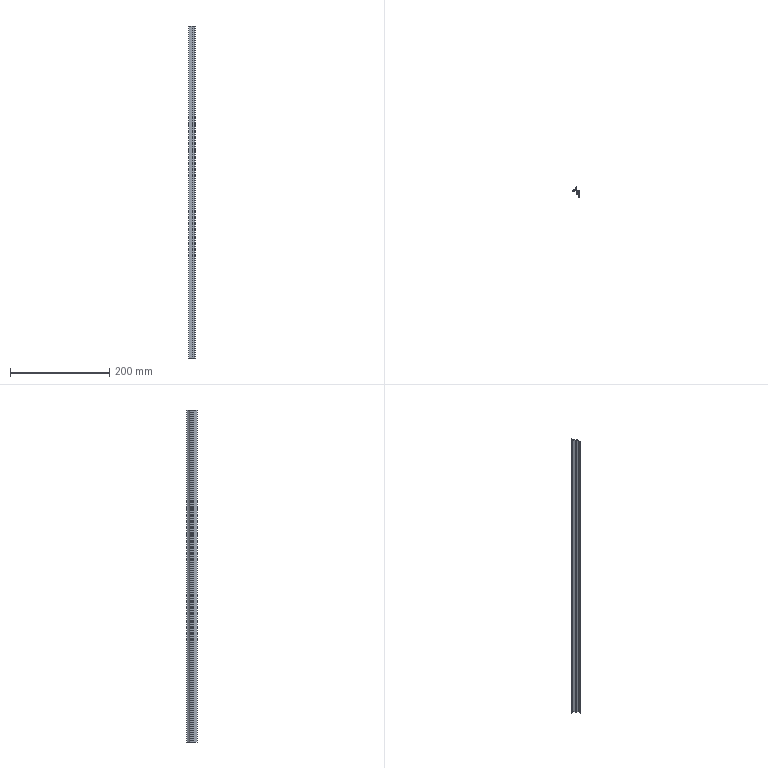Part | SolidWorks | features BaseBody 1, ICE 1, MoveFace 1 | 1 solid | 27 faces | box 14 x 20.3 x 670 mm | volume 34114 mm3 | plane 20 | cylinder 7 | commonest cylinder face diameters 0.387 x2 0.8 x2 0.4 x1 20 x1 22 x1
STEP:
#1=CARTESIAN_POINT('',(-5.304,-0.625,200.));
#2=VERTEX_POINT('',#1);
#3=CARTESIAN_POINT('',(-5.449,-0.8125,200.));
#4=VERTEX_POINT('',#3);
#5=CARTESIAN_POINT('',(-5.255,-0.8125,200.));
#6=DIRECTION('',(0.,0.,1.));
#7=DIRECTION('',(-1.,0.,0.));
#8=AXIS2_PLACEMENT_3D('',#5,#6,#7);
#9=CIRCLE('',#8,0.1937);
#10=EDGE_CURVE('',#2,#4,#9,.T.);
#11=ORIENTED_EDGE('',*,*,#10,.T.);
#12=CARTESIAN_POINT('',(-5.449,-0.8125,-470.));
#13=VERTEX_POINT('',#12);
#14=CARTESIAN_POINT('',(-5.449,-0.8125,230.));
#15=DIRECTION('',(0.,0.,-1.));
#16=VECTOR('',#15,1000.);
#17=LINE('',#14,#16);
#18=EDGE_CURVE('',#4,#13,#17,.T.);
#19=ORIENTED_EDGE('',*,*,#18,.T.);
#20=CARTESIAN_POINT('',(-5.304,-0.625,-470.));
#21=VERTEX_POINT('',#20);
#22=CARTESIAN_POINT('',(-5.255,-0.8125,-470.));
#23=DIRECTION('',(0.,0.,-1.));
#24=DIRECTION('',(1.,0.,0.));
#25=AXIS2_PLACEMENT_3D('',#22,#23,#24);
#26=CIRCLE('',#25,0.1937);
#27=EDGE_CURVE('',#13,#21,#26,.T.);
#28=ORIENTED_EDGE('',*,*,#27,.T.);
#29=CARTESIAN_POINT('',(-5.304,-0.625,230.));
#30=DIRECTION('',(0.,0.,-1.));
#31=VECTOR('',#30,1000.);
#32=LINE('',#29,#31);
#33=EDGE_CURVE('',#2,#21,#32,.T.);
#34=ORIENTED_EDGE('',*,*,#33,.F.);
#35=EDGE_LOOP('',(#11,#19,#28,#34));
#36=FACE_OUTER_BOUND('',#35,.T.);
#37=CARTESIAN_POINT('',(-5.255,-0.8125,230.));
#38=DIRECTION('',(0.,0.,-1.));
#39=DIRECTION('',(-1.,0.,0.));
#40=AXIS2_PLACEMENT_3D('',#37,#38,#39);
#41=CYLINDRICAL_SURFACE('',#40,0.1937);
#42=ADVANCED_FACE('',(#36),#41,.F.);
#43=CARTESIAN_POINT('',(5.,-1.,-470.));
#44=VERTEX_POINT('',#43);
#45=CARTESIAN_POINT('',(5.,-14.3,-470.));
#46=VERTEX_POINT('',#45);
#47=CARTESIAN_POINT('',(5.,29.623,-470.));
#48=DIRECTION('',(0.,-1.,0.));
#49=VECTOR('',#48,1000.);
#50=LINE('',#47,#49);
#51=EDGE_CURVE('',#44,#46,#50,.T.);
#52=ORIENTED_EDGE('',*,*,#51,.F.);
#53=CARTESIAN_POINT('',(5.,-1.,200.));
#54=VERTEX_POINT('',#53);
#55=CARTESIAN_POINT('',(5.,-1.,230.));
#56=DIRECTION('',(0.,0.,-1.));
#57=VECTOR('',#56,1000.);
#58=LINE('',#55,#57);
#59=EDGE_CURVE('',#54,#44,#58,.T.);
#60=ORIENTED_EDGE('',*,*,#59,.F.);
#61=CARTESIAN_POINT('',(5.,-14.3,200.));
#62=VERTEX_POINT('',#61);
#63=CARTESIAN_POINT('',(5.,-14.3,200.));
#64=DIRECTION('',(0.,1.,0.));
#65=VECTOR('',#64,1000.);
#66=LINE('',#63,#65);
#67=EDGE_CURVE('',#62,#54,#66,.T.);
#68=ORIENTED_EDGE('',*,*,#67,.F.);
#69=CARTESIAN_POINT('',(5.,-14.3,230.));
#70=DIRECTION('',(0.,0.,1.));
#71=VECTOR('',#70,1000.);
#72=LINE('',#69,#71);
#73=EDGE_CURVE('',#46,#62,#72,.T.);
#74=ORIENTED_EDGE('',*,*,#73,.F.);
#75=EDGE_LOOP('',(#52,#60,#68,#74));
#76=FACE_OUTER_BOUND('',#75,.T.);
#77=CARTESIAN_POINT('',(5.,-14.3,230.));
#78=DIRECTION('',(-1.,0.,0.));
#79=DIRECTION('',(0.,0.,1.));
#80=AXIS2_PLACEMENT_3D('',#77,#78,#79);
#81=PLANE('',#80);
#82=ADVANCED_FACE('',(#76),#81,.F.);
#83=CARTESIAN_POINT('',(-9.,-2.,-470.));
#84=VERTEX_POINT('',#83);
#85=CARTESIAN_POINT('',(-9.,-2.,200.));
#86=VERTEX_POINT('',#85);
#87=CARTESIAN_POINT('',(-9.,-2.,230.));
#88=DIRECTION('',(0.,0.,1.));
#89=VECTOR('',#88,1000.);
#90=LINE('',#87,#89);
#91=EDGE_CURVE('',#84,#86,#90,.T.);
#92=ORIENTED_EDGE('',*,*,#91,.F.);
#93=CARTESIAN_POINT('',(0.9,-2.,-470.));
#94=VERTEX_POINT('',#93);
#95=CARTESIAN_POINT('',(5.,-2.,-470.));
#96=DIRECTION('',(-1.,0.,0.));
#97=VECTOR('',#96,1000.);
#98=LINE('',#95,#97);
#99=EDGE_CURVE('',#94,#84,#98,.T.);
#100=ORIENTED_EDGE('',*,*,#99,.F.);
#101=CARTESIAN_POINT('',(0.9,-2.,200.));
#102=VERTEX_POINT('',#101);
#103=CARTESIAN_POINT('',(0.9,-2.,230.));
#104=DIRECTION('',(0.,0.,-1.));
#105=VECTOR('',#104,1000.);
#106=LINE('',#103,#105);
#107=EDGE_CURVE('',#102,#94,#106,.T.);
#108=ORIENTED_EDGE('',*,*,#107,.F.);
#109=CARTESIAN_POINT('',(5.,-2.,200.));
#110=DIRECTION('',(1.,0.,0.));
#111=VECTOR('',#110,1000.);
#112=LINE('',#109,#111);
#113=EDGE_CURVE('',#86,#102,#112,.T.);
#114=ORIENTED_EDGE('',*,*,#113,.F.);
#115=EDGE_LOOP('',(#92,#100,#108,#114));
#116=FACE_OUTER_BOUND('',#115,.T.);
#117=CARTESIAN_POINT('',(-9.,-2.,230.));
#118=DIRECTION('',(0.,1.,0.));
#119=DIRECTION('',(0.,0.,1.));
#120=AXIS2_PLACEMENT_3D('',#117,#118,#119);
#121=PLANE('',#120);
#122=ADVANCED_FACE('',(#116),#121,.F.);
#123=CARTESIAN_POINT('',(4.,-6.,200.));
#124=VERTEX_POINT('',#123);
#125=CARTESIAN_POINT('',(4.,-3.,200.));
#126=VERTEX_POINT('',#125);
#127=CARTESIAN_POINT('',(4.,29.623,200.));
#128=DIRECTION('',(0.,1.,0.));
#129=VECTOR('',#128,1000.);
#130=LINE('',#127,#129);
#131=EDGE_CURVE('',#124,#126,#130,.T.);
#132=ORIENTED_EDGE('',*,*,#131,.F.);
#133=CARTESIAN_POINT('',(1.,-6.,200.));
#134=VERTEX_POINT('',#133);
#135=CARTESIAN_POINT('',(5.,-6.,200.));
#136=DIRECTION('',(1.,0.,0.));
#137=VECTOR('',#136,1000.);
#138=LINE('',#135,#137);
#139=EDGE_CURVE('',#134,#124,#138,.T.);
#140=ORIENTED_EDGE('',*,*,#139,.F.);
#141=CARTESIAN_POINT('',(1.,-6.7,200.));
#142=VERTEX_POINT('',#141);
#143=CARTESIAN_POINT('',(1.,-6.,200.));
#144=DIRECTION('',(0.,-1.,0.));
#145=VECTOR('',#144,1000.);
#146=LINE('',#143,#145);
#147=EDGE_CURVE('',#134,#142,#146,.T.);
#148=ORIENTED_EDGE('',*,*,#147,.T.);
#149=CARTESIAN_POINT('',(-1.7,-6.7,200.));
#150=VERTEX_POINT('',#149);
#151=CARTESIAN_POINT('',(5.,-6.7,200.));
#152=DIRECTION('',(1.,0.,0.));
#153=VECTOR('',#152,1000.);
#154=LINE('',#151,#153);
#155=EDGE_CURVE('',#150,#142,#154,.T.);
#156=ORIENTED_EDGE('',*,*,#155,.F.);
#157=CARTESIAN_POINT('',(-1.7,-7.7,200.));
#158=VERTEX_POINT('',#157);
#159=CARTESIAN_POINT('',(-1.7,-6.7,200.));
#160=DIRECTION('',(0.,-1.,0.));
#161=VECTOR('',#160,1000.);
#162=LINE('',#159,#161);
#163=EDGE_CURVE('',#150,#158,#162,.T.);
#164=ORIENTED_EDGE('',*,*,#163,.T.);
#165=CARTESIAN_POINT('',(4.,-7.7,200.));
#166=VERTEX_POINT('',#165);
#167=CARTESIAN_POINT('',(5.,-7.7,200.));
#168=DIRECTION('',(-1.,0.,0.));
#169=VECTOR('',#168,1000.);
#170=LINE('',#167,#169);
#171=EDGE_CURVE('',#166,#158,#170,.T.);
#172=ORIENTED_EDGE('',*,*,#171,.F.);
#173=CARTESIAN_POINT('',(4.,-14.3,200.));
#174=VERTEX_POINT('',#173);
#175=CARTESIAN_POINT('',(4.,29.623,200.));
#176=DIRECTION('',(0.,1.,0.));
#177=VECTOR('',#176,1000.);
#178=LINE('',#175,#177);
#179=EDGE_CURVE('',#174,#166,#178,.T.);
#180=ORIENTED_EDGE('',*,*,#179,.F.);
#181=CARTESIAN_POINT('',(5.,-14.3,200.));
#182=DIRECTION('',(-1.,0.,0.));
#183=VECTOR('',#182,1000.);
#184=LINE('',#181,#183);
#185=EDGE_CURVE('',#62,#174,#184,.T.);
#186=ORIENTED_EDGE('',*,*,#185,.F.);
#187=ORIENTED_EDGE('',*,*,#67,.T.);
#188=CARTESIAN_POINT('',(-5.207,-1.,200.));
#189=VERTEX_POINT('',#188);
#190=CARTESIAN_POINT('',(5.,-1.,200.));
#191=DIRECTION('',(1.,0.,0.));
#192=VECTOR('',#191,1000.);
#193=LINE('',#190,#192);
#194=EDGE_CURVE('',#189,#54,#193,.T.);
#195=ORIENTED_EDGE('',*,*,#194,.F.);
#196=CARTESIAN_POINT('',(-5.255,-0.8125,200.));
#197=DIRECTION('',(0.,0.,1.));
#198=DIRECTION('',(-1.,0.,0.));
#199=AXIS2_PLACEMENT_3D('',#196,#197,#198);
#200=CIRCLE('',#199,0.1937);
#201=EDGE_CURVE('',#4,#189,#200,.T.);
#202=ORIENTED_EDGE('',*,*,#201,.F.);
#203=ORIENTED_EDGE('',*,*,#10,.F.);
#204=CARTESIAN_POINT('',(-1.368,3.063,200.));
#205=VERTEX_POINT('',#204);
#206=CARTESIAN_POINT('',(-10.628,9.,200.));
#207=DIRECTION('',(0.,0.,1.));
#208=DIRECTION('',(-1.,0.,0.));
#209=AXIS2_PLACEMENT_3D('',#206,#207,#208);
#210=CIRCLE('',#209,11.);
#211=EDGE_CURVE('',#2,#205,#210,.T.);
#212=ORIENTED_EDGE('',*,*,#211,.T.);
#213=CARTESIAN_POINT('',(-1.,2.955,200.));
#214=VERTEX_POINT('',#213);
#215=CARTESIAN_POINT('',(-1.2,2.955,200.));
#216=DIRECTION('',(0.,0.,1.));
#217=DIRECTION('',(-1.,0.,0.));
#218=AXIS2_PLACEMENT_3D('',#215,#216,#217);
#219=CIRCLE('',#218,0.2);
#220=EDGE_CURVE('',#214,#205,#219,.T.);
#221=ORIENTED_EDGE('',*,*,#220,.F.);
#222=CARTESIAN_POINT('',(-1.,1.5,200.));
#223=VERTEX_POINT('',#222);
#224=CARTESIAN_POINT('',(-1.,2.955,200.));
#225=DIRECTION('',(0.,1.,0.));
#226=VECTOR('',#225,1000.);
#227=LINE('',#224,#226);
#228=EDGE_CURVE('',#223,#214,#227,.T.);
#229=ORIENTED_EDGE('',*,*,#228,.F.);
#230=CARTESIAN_POINT('',(0.,1.5,200.));
#231=VERTEX_POINT('',#230);
#232=CARTESIAN_POINT('',(-1.,1.5,200.));
#233=DIRECTION('',(-1.,0.,0.));
#234=VECTOR('',#233,1000.);
#235=LINE('',#232,#234);
#236=EDGE_CURVE('',#231,#223,#235,.T.);
#237=ORIENTED_EDGE('',*,*,#236,.F.);
#238=CARTESIAN_POINT('',(0.,6.,200.));
#239=VERTEX_POINT('',#238);
#240=CARTESIAN_POINT('',(0.,1.5,200.));
#241=DIRECTION('',(0.,-1.,0.));
#242=VECTOR('',#241,1000.);
#243=LINE('',#240,#242);
#244=EDGE_CURVE('',#239,#231,#243,.T.);
#245=ORIENTED_EDGE('',*,*,#244,.F.);
#246=CARTESIAN_POINT('',(-0.8,6.,200.));
#247=VERTEX_POINT('',#246);
#248=CARTESIAN_POINT('',(0.,6.,200.));
#249=DIRECTION('',(1.,0.,0.));
#250=VECTOR('',#249,1000.);
#251=LINE('',#248,#250);
#252=EDGE_CURVE('',#247,#239,#251,.T.);
#253=ORIENTED_EDGE('',*,*,#252,.F.);
#254=CARTESIAN_POINT('',(-1.178,5.731,200.));
#255=VERTEX_POINT('',#254);
#256=CARTESIAN_POINT('',(-0.8,5.6,200.));
#257=DIRECTION('',(0.,0.,1.));
#258=DIRECTION('',(-1.,0.,0.));
#259=AXIS2_PLACEMENT_3D('',#256,#257,#258);
#260=CIRCLE('',#259,0.4);
#261=EDGE_CURVE('',#247,#255,#260,.T.);
#262=ORIENTED_EDGE('',*,*,#261,.T.);
#263=CARTESIAN_POINT('',(-8.678,-0.8077,200.));
#264=VERTEX_POINT('',#263);
#265=CARTESIAN_POINT('',(-10.628,9.,200.));
#266=DIRECTION('',(0.,0.,1.));
#267=DIRECTION('',(-1.,0.,0.));
#268=AXIS2_PLACEMENT_3D('',#265,#266,#267);
#269=CIRCLE('',#268,10.);
#270=EDGE_CURVE('',#264,#255,#269,.T.);
#271=ORIENTED_EDGE('',*,*,#270,.F.);
#272=CARTESIAN_POINT('',(-9.,-1.2,200.));
#273=VERTEX_POINT('',#272);
#274=CARTESIAN_POINT('',(-8.6,-1.2,200.));
#275=DIRECTION('',(0.,0.,1.));
#276=DIRECTION('',(-1.,0.,0.));
#277=AXIS2_PLACEMENT_3D('',#274,#275,#276);
#278=CIRCLE('',#277,0.4);
#279=EDGE_CURVE('',#264,#273,#278,.T.);
#280=ORIENTED_EDGE('',*,*,#279,.T.);
#281=CARTESIAN_POINT('',(-9.,8.,200.));
#282=DIRECTION('',(0.,-1.,0.));
#283=VECTOR('',#282,1000.);
#284=LINE('',#281,#283);
#285=EDGE_CURVE('',#273,#86,#284,.T.);
#286=ORIENTED_EDGE('',*,*,#285,.T.);
#287=ORIENTED_EDGE('',*,*,#113,.T.);
#288=CARTESIAN_POINT('',(0.9,-3.,200.));
#289=VERTEX_POINT('',#288);
#290=CARTESIAN_POINT('',(0.9,29.623,200.));
#291=DIRECTION('',(0.,1.,0.));
#292=VECTOR('',#291,1000.);
#293=LINE('',#290,#292);
#294=EDGE_CURVE('',#289,#102,#293,.T.);
#295=ORIENTED_EDGE('',*,*,#294,.F.);
#296=CARTESIAN_POINT('',(5.,-3.,200.));
#297=DIRECTION('',(-1.,0.,0.));
#298=VECTOR('',#297,1000.);
#299=LINE('',#296,#298);
#300=EDGE_CURVE('',#126,#289,#299,.T.);
#301=ORIENTED_EDGE('',*,*,#300,.F.);
#302=EDGE_LOOP('',(#132,#140,#148,#156,#164,#172,#180,#186,#187,#195,#202,#203,#212,#221,#229,#237,#245,#253,#262,#271,#280,#286,#287,#295,#301));
#303=FACE_OUTER_BOUND('',#302,.T.);
#304=CARTESIAN_POINT('',(5.,29.623,200.));
#305=DIRECTION('',(0.,0.,-1.));
#306=DIRECTION('',(-1.,0.,0.));
#307=AXIS2_PLACEMENT_3D('',#304,#305,#306);
#308=PLANE('',#307);
#309=ADVANCED_FACE('',(#303),#308,.F.);
#310=ORIENTED_EDGE('',*,*,#185,.T.);
#311=CARTESIAN_POINT('',(4.,-14.3,-470.));
#312=VERTEX_POINT('',#311);
#313=CARTESIAN_POINT('',(4.,-14.3,230.));
#314=DIRECTION('',(0.,0.,1.));
#315=VECTOR('',#314,1000.);
#316=LINE('',#313,#315);
#317=EDGE_CURVE('',#312,#174,#316,.T.);
#318=ORIENTED_EDGE('',*,*,#317,.F.);
#319=CARTESIAN_POINT('',(5.,-14.3,-470.));
#320=DIRECTION('',(-1.,0.,0.));
#321=VECTOR('',#320,1000.);
#322=LINE('',#319,#321);
#323=EDGE_CURVE('',#46,#312,#322,.T.);
#324=ORIENTED_EDGE('',*,*,#323,.F.);
#325=ORIENTED_EDGE('',*,*,#73,.T.);
#326=EDGE_LOOP('',(#310,#318,#324,#325));
#327=FACE_OUTER_BOUND('',#326,.T.);
#328=CARTESIAN_POINT('',(4.,-14.3,230.));
#329=DIRECTION('',(0.,1.,0.));
#330=DIRECTION('',(0.,0.,1.));
#331=AXIS2_PLACEMENT_3D('',#328,#329,#330);
#332=PLANE('',#331);
#333=ADVANCED_FACE('',(#327),#332,.F.);
#334=ORIENTED_EDGE('',*,*,#51,.T.);
#335=ORIENTED_EDGE('',*,*,#323,.T.);
#336=CARTESIAN_POINT('',(4.,-7.7,-470.));
#337=VERTEX_POINT('',#336);
#338=CARTESIAN_POINT('',(4.,-7.7,-470.));
#339=DIRECTION('',(0.,-1.,0.));
#340=VECTOR('',#339,1000.);
#341=LINE('',#338,#340);
#342=EDGE_CURVE('',#337,#312,#341,.T.);
#343=ORIENTED_EDGE('',*,*,#342,.F.);
#344=CARTESIAN_POINT('',(-1.7,-7.7,-470.));
#345=VERTEX_POINT('',#344);
#346=CARTESIAN_POINT('',(-1.7,-7.7,-470.));
#347=DIRECTION('',(1.,0.,0.));
#348=VECTOR('',#347,1000.);
#349=LINE('',#346,#348);
#350=EDGE_CURVE('',#345,#337,#349,.T.);
#351=ORIENTED_EDGE('',*,*,#350,.F.);
#352=CARTESIAN_POINT('',(-1.7,-6.7,-470.));
#353=VERTEX_POINT('',#352);
#354=CARTESIAN_POINT('',(-1.7,29.623,-470.));
#355=DIRECTION('',(0.,1.,0.));
#356=VECTOR('',#355,1000.);
#357=LINE('',#354,#356);
#358=EDGE_CURVE('',#345,#353,#357,.T.);
#359=ORIENTED_EDGE('',*,*,#358,.T.);
#360=CARTESIAN_POINT('',(1.,-6.7,-470.));
#361=VERTEX_POINT('',#360);
#362=CARTESIAN_POINT('',(1.,-6.7,-470.));
#363=DIRECTION('',(-1.,0.,0.));
#364=VECTOR('',#363,1000.);
#365=LINE('',#362,#364);
#366=EDGE_CURVE('',#361,#353,#365,.T.);
#367=ORIENTED_EDGE('',*,*,#366,.F.);
#368=CARTESIAN_POINT('',(1.,-6.,-470.));
#369=VERTEX_POINT('',#368);
#370=CARTESIAN_POINT('',(1.,29.623,-470.));
#371=DIRECTION('',(0.,1.,0.));
#372=VECTOR('',#371,1000.);
#373=LINE('',#370,#372);
#374=EDGE_CURVE('',#361,#369,#373,.T.);
#375=ORIENTED_EDGE('',*,*,#374,.T.);
#376=CARTESIAN_POINT('',(4.,-6.,-470.));
#377=VERTEX_POINT('',#376);
#378=CARTESIAN_POINT('',(4.,-6.,-470.));
#379=DIRECTION('',(-1.,0.,0.));
#380=VECTOR('',#379,1000.);
#381=LINE('',#378,#380);
#382=EDGE_CURVE('',#377,#369,#381,.T.);
#383=ORIENTED_EDGE('',*,*,#382,.F.);
#384=CARTESIAN_POINT('',(4.,-3.,-470.));
#385=VERTEX_POINT('',#384);
#386=CARTESIAN_POINT('',(4.,-3.,-470.));
#387=DIRECTION('',(0.,-1.,0.));
#388=VECTOR('',#387,1000.);
#389=LINE('',#386,#388);
#390=EDGE_CURVE('',#385,#377,#389,.T.);
#391=ORIENTED_EDGE('',*,*,#390,.F.);
#392=CARTESIAN_POINT('',(0.9,-3.,-470.));
#393=VERTEX_POINT('',#392);
#394=CARTESIAN_POINT('',(0.9,-3.,-470.));
#395=DIRECTION('',(1.,0.,0.));
#396=VECTOR('',#395,1000.);
#397=LINE('',#394,#396);
#398=EDGE_CURVE('',#393,#385,#397,.T.);
#399=ORIENTED_EDGE('',*,*,#398,.F.);
#400=CARTESIAN_POINT('',(0.9,-2.,-470.));
#401=DIRECTION('',(0.,-1.,0.));
#402=VECTOR('',#401,1000.);
#403=LINE('',#400,#402);
#404=EDGE_CURVE('',#94,#393,#403,.T.);
#405=ORIENTED_EDGE('',*,*,#404,.F.);
#406=ORIENTED_EDGE('',*,*,#99,.T.);
#407=CARTESIAN_POINT('',(-9.,-1.2,-470.));
#408=VERTEX_POINT('',#407);
#409=CARTESIAN_POINT('',(-9.,-1.2,-470.));
#410=DIRECTION('',(0.,-1.,0.));
#411=VECTOR('',#410,1000.);
#412=LINE('',#409,#411);
#413=EDGE_CURVE('',#408,#84,#412,.T.);
#414=ORIENTED_EDGE('',*,*,#413,.F.);
#415=CARTESIAN_POINT('',(-8.678,-0.8077,-470.));
#416=VERTEX_POINT('',#415);
#417=CARTESIAN_POINT('',(-8.6,-1.2,-470.));
#418=DIRECTION('',(0.,0.,-1.));
#419=DIRECTION('',(1.,0.,0.));
#420=AXIS2_PLACEMENT_3D('',#417,#418,#419);
#421=CIRCLE('',#420,0.4);
#422=EDGE_CURVE('',#408,#416,#421,.T.);
#423=ORIENTED_EDGE('',*,*,#422,.T.);
#424=CARTESIAN_POINT('',(-1.178,5.731,-470.));
#425=VERTEX_POINT('',#424);
#426=CARTESIAN_POINT('',(-10.628,9.,-470.));
#427=DIRECTION('',(0.,0.,-1.));
#428=DIRECTION('',(1.,0.,0.));
#429=AXIS2_PLACEMENT_3D('',#426,#427,#428);
#430=CIRCLE('',#429,10.);
#431=EDGE_CURVE('',#425,#416,#430,.T.);
#432=ORIENTED_EDGE('',*,*,#431,.F.);
#433=CARTESIAN_POINT('',(-0.8,6.,-470.));
#434=VERTEX_POINT('',#433);
#435=CARTESIAN_POINT('',(-0.8,5.6,-470.));
#436=DIRECTION('',(0.,0.,-1.));
#437=DIRECTION('',(1.,0.,0.));
#438=AXIS2_PLACEMENT_3D('',#435,#436,#437);
#439=CIRCLE('',#438,0.4);
#440=EDGE_CURVE('',#425,#434,#439,.T.);
#441=ORIENTED_EDGE('',*,*,#440,.T.);
#442=CARTESIAN_POINT('',(0.,6.,-470.));
#443=VERTEX_POINT('',#442);
#444=CARTESIAN_POINT('',(0.,6.,-470.));
#445=DIRECTION('',(-1.,0.,0.));
#446=VECTOR('',#445,1000.);
#447=LINE('',#444,#446);
#448=EDGE_CURVE('',#443,#434,#447,.T.);
#449=ORIENTED_EDGE('',*,*,#448,.F.);
#450=CARTESIAN_POINT('',(0.,1.5,-470.));
#451=VERTEX_POINT('',#450);
#452=CARTESIAN_POINT('',(0.,1.5,-470.));
#453=DIRECTION('',(0.,1.,0.));
#454=VECTOR('',#453,1000.);
#455=LINE('',#452,#454);
#456=EDGE_CURVE('',#451,#443,#455,.T.);
#457=ORIENTED_EDGE('',*,*,#456,.F.);
#458=CARTESIAN_POINT('',(-1.,1.5,-470.));
#459=VERTEX_POINT('',#458);
#460=CARTESIAN_POINT('',(-1.,1.5,-470.));
#461=DIRECTION('',(1.,0.,0.));
#462=VECTOR('',#461,1000.);
#463=LINE('',#460,#462);
#464=EDGE_CURVE('',#459,#451,#463,.T.);
#465=ORIENTED_EDGE('',*,*,#464,.F.);
#466=CARTESIAN_POINT('',(-1.,2.955,-470.));
#467=VERTEX_POINT('',#466);
#468=CARTESIAN_POINT('',(-1.,2.955,-470.));
#469=DIRECTION('',(0.,-1.,0.));
#470=VECTOR('',#469,1000.);
#471=LINE('',#468,#470);
#472=EDGE_CURVE('',#467,#459,#471,.T.);
#473=ORIENTED_EDGE('',*,*,#472,.F.);
#474=CARTESIAN_POINT('',(-1.368,3.063,-470.));
#475=VERTEX_POINT('',#474);
#476=CARTESIAN_POINT('',(-1.2,2.955,-470.));
#477=DIRECTION('',(0.,0.,-1.));
#478=DIRECTION('',(1.,0.,0.));
#479=AXIS2_PLACEMENT_3D('',#476,#477,#478);
#480=CIRCLE('',#479,0.2);
#481=EDGE_CURVE('',#475,#467,#480,.T.);
#482=ORIENTED_EDGE('',*,*,#481,.F.);
#483=CARTESIAN_POINT('',(-10.628,9.,-470.));
#484=DIRECTION('',(0.,0.,-1.));
#485=DIRECTION('',(1.,0.,0.));
#486=AXIS2_PLACEMENT_3D('',#483,#484,#485);
#487=CIRCLE('',#486,11.);
#488=EDGE_CURVE('',#475,#21,#487,.T.);
#489=ORIENTED_EDGE('',*,*,#488,.T.);
#490=ORIENTED_EDGE('',*,*,#27,.F.);
#491=CARTESIAN_POINT('',(-5.207,-1.,-470.));
#492=VERTEX_POINT('',#491);
#493=CARTESIAN_POINT('',(-5.255,-0.8125,-470.));
#494=DIRECTION('',(0.,0.,-1.));
#495=DIRECTION('',(1.,0.,0.));
#496=AXIS2_PLACEMENT_3D('',#493,#494,#495);
#497=CIRCLE('',#496,0.1937);
#498=EDGE_CURVE('',#492,#13,#497,.T.);
#499=ORIENTED_EDGE('',*,*,#498,.F.);
#500=CARTESIAN_POINT('',(5.,-1.,-470.));
#501=DIRECTION('',(-1.,0.,0.));
#502=VECTOR('',#501,1000.);
#503=LINE('',#500,#502);
#504=EDGE_CURVE('',#44,#492,#503,.T.);
#505=ORIENTED_EDGE('',*,*,#504,.F.);
#506=EDGE_LOOP('',(#334,#335,#343,#351,#359,#367,#375,#383,#391,#399,#405,#406,#414,#423,#432,#441,#449,#457,#465,#473,#482,#489,#490,#499,#505));
#507=FACE_OUTER_BOUND('',#506,.T.);
#508=CARTESIAN_POINT('',(5.,29.623,-470.));
#509=DIRECTION('',(0.,0.,1.));
#510=DIRECTION('',(1.,0.,0.));
#511=AXIS2_PLACEMENT_3D('',#508,#509,#510);
#512=PLANE('',#511);
#513=ADVANCED_FACE('',(#507),#512,.F.);
#514=ORIENTED_EDGE('',*,*,#59,.T.);
#515=ORIENTED_EDGE('',*,*,#504,.T.);
#516=CARTESIAN_POINT('',(-5.207,-1.,230.));
#517=DIRECTION('',(0.,0.,-1.));
#518=VECTOR('',#517,1000.);
#519=LINE('',#516,#518);
#520=EDGE_CURVE('',#189,#492,#519,.T.);
#521=ORIENTED_EDGE('',*,*,#520,.F.);
#522=ORIENTED_EDGE('',*,*,#194,.T.);
#523=EDGE_LOOP('',(#514,#515,#521,#522));
#524=FACE_OUTER_BOUND('',#523,.T.);
#525=CARTESIAN_POINT('',(5.,-1.,230.));
#526=DIRECTION('',(0.,-1.,0.));
#527=DIRECTION('',(0.,0.,-1.));
#528=AXIS2_PLACEMENT_3D('',#525,#526,#527);
#529=PLANE('',#528);
#530=ADVANCED_FACE('',(#524),#529,.F.);
#531=CARTESIAN_POINT('',(-9.,-1.2,230.));
#532=DIRECTION('',(0.,0.,1.));
#533=VECTOR('',#532,1000.);
#534=LINE('',#531,#533);
#535=EDGE_CURVE('',#408,#273,#534,.T.);
#536=ORIENTED_EDGE('',*,*,#535,.F.);
#537=ORIENTED_EDGE('',*,*,#413,.T.);
#538=ORIENTED_EDGE('',*,*,#91,.T.);
#539=ORIENTED_EDGE('',*,*,#285,.F.);
#540=EDGE_LOOP('',(#536,#537,#538,#539));
#541=FACE_OUTER_BOUND('',#540,.T.);
#542=CARTESIAN_POINT('',(-9.,-1.2,230.));
#543=DIRECTION('',(1.,0.,0.));
#544=DIRECTION('',(0.,0.,-1.));
#545=AXIS2_PLACEMENT_3D('',#542,#543,#544);
#546=PLANE('',#545);
#547=ADVANCED_FACE('',(#541),#546,.F.);
#548=ORIENTED_EDGE('',*,*,#294,.T.);
#549=ORIENTED_EDGE('',*,*,#107,.T.);
#550=ORIENTED_EDGE('',*,*,#404,.T.);
#551=CARTESIAN_POINT('',(0.9,-3.,230.));
#552=DIRECTION('',(0.,0.,-1.));
#553=VECTOR('',#552,1000.);
#554=LINE('',#551,#553);
#555=EDGE_CURVE('',#289,#393,#554,.T.);
#556=ORIENTED_EDGE('',*,*,#555,.F.);
#557=EDGE_LOOP('',(#548,#549,#550,#556));
#558=FACE_OUTER_BOUND('',#557,.T.);
#559=CARTESIAN_POINT('',(0.9,-2.,230.));
#560=DIRECTION('',(1.,0.,0.));
#561=DIRECTION('',(0.,0.,-1.));
#562=AXIS2_PLACEMENT_3D('',#559,#560,#561);
#563=PLANE('',#562);
#564=ADVANCED_FACE('',(#558),#563,.F.);
#565=ORIENTED_EDGE('',*,*,#300,.T.);
#566=ORIENTED_EDGE('',*,*,#555,.T.);
#567=ORIENTED_EDGE('',*,*,#398,.T.);
#568=CARTESIAN_POINT('',(4.,-3.,230.));
#569=DIRECTION('',(0.,0.,-1.));
#570=VECTOR('',#569,1000.);
#571=LINE('',#568,#570);
#572=EDGE_CURVE('',#126,#385,#571,.T.);
#573=ORIENTED_EDGE('',*,*,#572,.F.);
#574=EDGE_LOOP('',(#565,#566,#567,#573));
#575=FACE_OUTER_BOUND('',#574,.T.);
#576=CARTESIAN_POINT('',(0.9,-3.,230.));
#577=DIRECTION('',(0.,1.,0.));
#578=DIRECTION('',(0.,0.,1.));
#579=AXIS2_PLACEMENT_3D('',#576,#577,#578);
#580=PLANE('',#579);
#581=ADVANCED_FACE('',(#575),#580,.F.);
#582=ORIENTED_EDGE('',*,*,#131,.T.);
#583=ORIENTED_EDGE('',*,*,#572,.T.);
#584=ORIENTED_EDGE('',*,*,#390,.T.);
#585=CARTESIAN_POINT('',(4.,-6.,230.));
#586=DIRECTION('',(0.,0.,-1.));
#587=VECTOR('',#586,1000.);
#588=LINE('',#585,#587);
#589=EDGE_CURVE('',#124,#377,#588,.T.);
#590=ORIENTED_EDGE('',*,*,#589,.F.);
#591=EDGE_LOOP('',(#582,#583,#584,#590));
#592=FACE_OUTER_BOUND('',#591,.T.);
#593=CARTESIAN_POINT('',(4.,-3.,230.));
#594=DIRECTION('',(1.,0.,0.));
#595=DIRECTION('',(0.,0.,-1.));
#596=AXIS2_PLACEMENT_3D('',#593,#594,#595);
#597=PLANE('',#596);
#598=ADVANCED_FACE('',(#592),#597,.F.);
#599=ORIENTED_EDGE('',*,*,#139,.T.);
#600=ORIENTED_EDGE('',*,*,#589,.T.);
#601=ORIENTED_EDGE('',*,*,#382,.T.);
#602=CARTESIAN_POINT('',(1.,-6.,230.));
#603=DIRECTION('',(0.,0.,-1.));
#604=VECTOR('',#603,1000.);
#605=LINE('',#602,#604);
#606=EDGE_CURVE('',#134,#369,#605,.T.);
#607=ORIENTED_EDGE('',*,*,#606,.F.);
#608=EDGE_LOOP('',(#599,#600,#601,#607));
#609=FACE_OUTER_BOUND('',#608,.T.);
#610=CARTESIAN_POINT('',(4.,-6.,230.));
#611=DIRECTION('',(0.,-1.,0.));
#612=DIRECTION('',(0.,0.,-1.));
#613=AXIS2_PLACEMENT_3D('',#610,#611,#612);
#614=PLANE('',#613);
#615=ADVANCED_FACE('',(#609),#614,.F.);
#616=ORIENTED_EDGE('',*,*,#155,.T.);
#617=CARTESIAN_POINT('',(1.,-6.7,230.));
#618=DIRECTION('',(0.,0.,1.));
#619=VECTOR('',#618,1000.);
#620=LINE('',#617,#619);
#621=EDGE_CURVE('',#361,#142,#620,.T.);
#622=ORIENTED_EDGE('',*,*,#621,.F.);
#623=ORIENTED_EDGE('',*,*,#366,.T.);
#624=CARTESIAN_POINT('',(-1.7,-6.7,230.));
#625=DIRECTION('',(0.,0.,-1.));
#626=VECTOR('',#625,1000.);
#627=LINE('',#624,#626);
#628=EDGE_CURVE('',#150,#353,#627,.T.);
#629=ORIENTED_EDGE('',*,*,#628,.F.);
#630=EDGE_LOOP('',(#616,#622,#623,#629));
#631=FACE_OUTER_BOUND('',#630,.T.);
#632=CARTESIAN_POINT('',(1.,-6.7,230.));
#633=DIRECTION('',(0.,-1.,0.));
#634=DIRECTION('',(0.,0.,-1.));
#635=AXIS2_PLACEMENT_3D('',#632,#633,#634);
#636=PLANE('',#635);
#637=ADVANCED_FACE('',(#631),#636,.F.);
#638=ORIENTED_EDGE('',*,*,#171,.T.);
#639=CARTESIAN_POINT('',(-1.7,-7.7,230.));
#640=DIRECTION('',(0.,0.,1.));
#641=VECTOR('',#640,1000.);
#642=LINE('',#639,#641);
#643=EDGE_CURVE('',#345,#158,#642,.T.);
#644=ORIENTED_EDGE('',*,*,#643,.F.);
#645=ORIENTED_EDGE('',*,*,#350,.T.);
#646=CARTESIAN_POINT('',(4.,-7.7,230.));
#647=DIRECTION('',(0.,0.,-1.));
#648=VECTOR('',#647,1000.);
#649=LINE('',#646,#648);
#650=EDGE_CURVE('',#166,#337,#649,.T.);
#651=ORIENTED_EDGE('',*,*,#650,.F.);
#652=EDGE_LOOP('',(#638,#644,#645,#651));
#653=FACE_OUTER_BOUND('',#652,.T.);
#654=CARTESIAN_POINT('',(-1.7,-7.7,230.));
#655=DIRECTION('',(0.,1.,0.));
#656=DIRECTION('',(0.,0.,1.));
#657=AXIS2_PLACEMENT_3D('',#654,#655,#656);
#658=PLANE('',#657);
#659=ADVANCED_FACE('',(#653),#658,.F.);
#660=ORIENTED_EDGE('',*,*,#179,.T.);
#661=ORIENTED_EDGE('',*,*,#650,.T.);
#662=ORIENTED_EDGE('',*,*,#342,.T.);
#663=ORIENTED_EDGE('',*,*,#317,.T.);
#664=EDGE_LOOP('',(#660,#661,#662,#663));
#665=FACE_OUTER_BOUND('',#664,.T.);
#666=CARTESIAN_POINT('',(4.,-7.7,230.));
#667=DIRECTION('',(1.,0.,0.));
#668=DIRECTION('',(0.,0.,-1.));
#669=AXIS2_PLACEMENT_3D('',#666,#667,#668);
#670=PLANE('',#669);
#671=ADVANCED_FACE('',(#665),#670,.F.);
#672=ORIENTED_EDGE('',*,*,#18,.F.);
#673=ORIENTED_EDGE('',*,*,#201,.T.);
#674=ORIENTED_EDGE('',*,*,#520,.T.);
#675=ORIENTED_EDGE('',*,*,#498,.T.);
#676=EDGE_LOOP('',(#672,#673,#674,#675));
#677=FACE_OUTER_BOUND('',#676,.T.);
#678=CARTESIAN_POINT('',(-5.255,-0.8125,230.));
#679=DIRECTION('',(0.,0.,-1.));
#680=DIRECTION('',(-1.,0.,0.));
#681=AXIS2_PLACEMENT_3D('',#678,#679,#680);
#682=CYLINDRICAL_SURFACE('',#681,0.1937);
#683=ADVANCED_FACE('',(#677),#682,.F.);
#684=CARTESIAN_POINT('',(-1.,2.955,230.));
#685=DIRECTION('',(0.,0.,1.));
#686=VECTOR('',#685,1000.);
#687=LINE('',#684,#686);
#688=EDGE_CURVE('',#467,#214,#687,.T.);
#689=ORIENTED_EDGE('',*,*,#688,.F.);
#690=ORIENTED_EDGE('',*,*,#472,.T.);
#691=CARTESIAN_POINT('',(-1.,1.5,230.));
#692=DIRECTION('',(0.,0.,-1.));
#693=VECTOR('',#692,1000.);
#694=LINE('',#691,#693);
#695=EDGE_CURVE('',#223,#459,#694,.T.);
#696=ORIENTED_EDGE('',*,*,#695,.F.);
#697=ORIENTED_EDGE('',*,*,#228,.T.);
#698=EDGE_LOOP('',(#689,#690,#696,#697));
#699=FACE_OUTER_BOUND('',#698,.T.);
#700=CARTESIAN_POINT('',(-1.,2.955,230.));
#701=DIRECTION('',(1.,0.,0.));
#702=DIRECTION('',(0.,0.,-1.));
#703=AXIS2_PLACEMENT_3D('',#700,#701,#702);
#704=PLANE('',#703);
#705=ADVANCED_FACE('',(#699),#704,.F.);
#706=ORIENTED_EDGE('',*,*,#488,.F.);
#707=CARTESIAN_POINT('',(-1.368,3.063,230.));
#708=DIRECTION('',(0.,0.,1.));
#709=VECTOR('',#708,1000.);
#710=LINE('',#707,#709);
#711=EDGE_CURVE('',#475,#205,#710,.T.);
#712=ORIENTED_EDGE('',*,*,#711,.T.);
#713=ORIENTED_EDGE('',*,*,#211,.F.);
#714=ORIENTED_EDGE('',*,*,#33,.T.);
#715=EDGE_LOOP('',(#706,#712,#713,#714));
#716=FACE_OUTER_BOUND('',#715,.T.);
#717=CARTESIAN_POINT('',(-10.628,9.,230.));
#718=DIRECTION('',(0.,0.,-1.));
#719=DIRECTION('',(-1.,0.,0.));
#720=AXIS2_PLACEMENT_3D('',#717,#718,#719);
#721=CYLINDRICAL_SURFACE('',#720,11.);
#722=ADVANCED_FACE('',(#716),#721,.T.);
#723=CARTESIAN_POINT('',(-1.178,5.731,230.));
#724=DIRECTION('',(0.,0.,1.));
#725=VECTOR('',#724,1000.);
#726=LINE('',#723,#725);
#727=EDGE_CURVE('',#425,#255,#726,.T.);
#728=ORIENTED_EDGE('',*,*,#727,.F.);
#729=ORIENTED_EDGE('',*,*,#431,.T.);
#730=CARTESIAN_POINT('',(-8.678,-0.8077,230.));
#731=DIRECTION('',(0.,0.,-1.));
#732=VECTOR('',#731,1000.);
#733=LINE('',#730,#732);
#734=EDGE_CURVE('',#264,#416,#733,.T.);
#735=ORIENTED_EDGE('',*,*,#734,.F.);
#736=ORIENTED_EDGE('',*,*,#270,.T.);
#737=EDGE_LOOP('',(#728,#729,#735,#736));
#738=FACE_OUTER_BOUND('',#737,.T.);
#739=CARTESIAN_POINT('',(-10.628,9.,230.));
#740=DIRECTION('',(0.,0.,-1.));
#741=DIRECTION('',(-1.,0.,0.));
#742=AXIS2_PLACEMENT_3D('',#739,#740,#741);
#743=CYLINDRICAL_SURFACE('',#742,10.);
#744=ADVANCED_FACE('',(#738),#743,.F.);
#745=CARTESIAN_POINT('',(0.,1.5,230.));
#746=DIRECTION('',(0.,0.,1.));
#747=VECTOR('',#746,1000.);
#748=LINE('',#745,#747);
#749=EDGE_CURVE('',#451,#231,#748,.T.);
#750=ORIENTED_EDGE('',*,*,#749,.F.);
#751=ORIENTED_EDGE('',*,*,#456,.T.);
#752=CARTESIAN_POINT('',(0.,6.,230.));
#753=DIRECTION('',(0.,0.,-1.));
#754=VECTOR('',#753,1000.);
#755=LINE('',#752,#754);
#756=EDGE_CURVE('',#239,#443,#755,.T.);
#757=ORIENTED_EDGE('',*,*,#756,.F.);
#758=ORIENTED_EDGE('',*,*,#244,.T.);
#759=EDGE_LOOP('',(#750,#751,#757,#758));
#760=FACE_OUTER_BOUND('',#759,.T.);
#761=CARTESIAN_POINT('',(0.,1.5,230.));
#762=DIRECTION('',(-1.,0.,0.));
#763=DIRECTION('',(0.,0.,1.));
#764=AXIS2_PLACEMENT_3D('',#761,#762,#763);
#765=PLANE('',#764);
#766=ADVANCED_FACE('',(#760),#765,.F.);
#767=ORIENTED_EDGE('',*,*,#422,.F.);
#768=ORIENTED_EDGE('',*,*,#535,.T.);
#769=ORIENTED_EDGE('',*,*,#279,.F.);
#770=ORIENTED_EDGE('',*,*,#734,.T.);
#771=EDGE_LOOP('',(#767,#768,#769,#770));
#772=FACE_OUTER_BOUND('',#771,.T.);
#773=CARTESIAN_POINT('',(-8.6,-1.2,230.));
#774=DIRECTION('',(0.,0.,-1.));
#775=DIRECTION('',(-1.,0.,0.));
#776=AXIS2_PLACEMENT_3D('',#773,#774,#775);
#777=CYLINDRICAL_SURFACE('',#776,0.4);
#778=ADVANCED_FACE('',(#772),#777,.T.);
#779=ORIENTED_EDGE('',*,*,#147,.F.);
#780=ORIENTED_EDGE('',*,*,#606,.T.);
#781=ORIENTED_EDGE('',*,*,#374,.F.);
#782=ORIENTED_EDGE('',*,*,#621,.T.);
#783=EDGE_LOOP('',(#779,#780,#781,#782));
#784=FACE_OUTER_BOUND('',#783,.T.);
#785=CARTESIAN_POINT('',(1.,-6.,230.));
#786=DIRECTION('',(1.,0.,0.));
#787=DIRECTION('',(0.,0.,-1.));
#788=AXIS2_PLACEMENT_3D('',#785,#786,#787);
#789=PLANE('',#788);
#790=ADVANCED_FACE('',(#784),#789,.F.);
#791=ORIENTED_EDGE('',*,*,#163,.F.);
#792=ORIENTED_EDGE('',*,*,#628,.T.);
#793=ORIENTED_EDGE('',*,*,#358,.F.);
#794=ORIENTED_EDGE('',*,*,#643,.T.);
#795=EDGE_LOOP('',(#791,#792,#793,#794));
#796=FACE_OUTER_BOUND('',#795,.T.);
#797=CARTESIAN_POINT('',(-1.7,-6.7,230.));
#798=DIRECTION('',(1.,0.,0.));
#799=DIRECTION('',(0.,0.,-1.));
#800=AXIS2_PLACEMENT_3D('',#797,#798,#799);
#801=PLANE('',#800);
#802=ADVANCED_FACE('',(#796),#801,.F.);
#803=ORIENTED_EDGE('',*,*,#711,.F.);
#804=ORIENTED_EDGE('',*,*,#481,.T.);
#805=ORIENTED_EDGE('',*,*,#688,.T.);
#806=ORIENTED_EDGE('',*,*,#220,.T.);
#807=EDGE_LOOP('',(#803,#804,#805,#806));
#808=FACE_OUTER_BOUND('',#807,.T.);
#809=CARTESIAN_POINT('',(-1.2,2.955,230.));
#810=DIRECTION('',(0.,0.,-1.));
#811=DIRECTION('',(-1.,0.,0.));
#812=AXIS2_PLACEMENT_3D('',#809,#810,#811);
#813=CYLINDRICAL_SURFACE('',#812,0.2);
#814=ADVANCED_FACE('',(#808),#813,.F.);
#815=ORIENTED_EDGE('',*,*,#695,.T.);
#816=ORIENTED_EDGE('',*,*,#464,.T.);
#817=ORIENTED_EDGE('',*,*,#749,.T.);
#818=ORIENTED_EDGE('',*,*,#236,.T.);
#819=EDGE_LOOP('',(#815,#816,#817,#818));
#820=FACE_OUTER_BOUND('',#819,.T.);
#821=CARTESIAN_POINT('',(-1.,1.5,230.));
#822=DIRECTION('',(0.,1.,0.));
#823=DIRECTION('',(0.,0.,1.));
#824=AXIS2_PLACEMENT_3D('',#821,#822,#823);
#825=PLANE('',#824);
#826=ADVANCED_FACE('',(#820),#825,.F.);
#827=ORIENTED_EDGE('',*,*,#440,.F.);
#828=ORIENTED_EDGE('',*,*,#727,.T.);
#829=ORIENTED_EDGE('',*,*,#261,.F.);
#830=CARTESIAN_POINT('',(-0.8,6.,230.));
#831=DIRECTION('',(0.,0.,-1.));
#832=VECTOR('',#831,1000.);
#833=LINE('',#830,#832);
#834=EDGE_CURVE('',#247,#434,#833,.T.);
#835=ORIENTED_EDGE('',*,*,#834,.T.);
#836=EDGE_LOOP('',(#827,#828,#829,#835));
#837=FACE_OUTER_BOUND('',#836,.T.);
#838=CARTESIAN_POINT('',(-0.8,5.6,230.));
#839=DIRECTION('',(0.,0.,-1.));
#840=DIRECTION('',(-1.,0.,0.));
#841=AXIS2_PLACEMENT_3D('',#838,#839,#840);
#842=CYLINDRICAL_SURFACE('',#841,0.4);
#843=ADVANCED_FACE('',(#837),#842,.T.);
#844=ORIENTED_EDGE('',*,*,#756,.T.);
#845=ORIENTED_EDGE('',*,*,#448,.T.);
#846=ORIENTED_EDGE('',*,*,#834,.F.);
#847=ORIENTED_EDGE('',*,*,#252,.T.);
#848=EDGE_LOOP('',(#844,#845,#846,#847));
#849=FACE_OUTER_BOUND('',#848,.T.);
#850=CARTESIAN_POINT('',(0.,6.,230.));
#851=DIRECTION('',(0.,-1.,0.));
#852=DIRECTION('',(0.,0.,-1.));
#853=AXIS2_PLACEMENT_3D('',#850,#851,#852);
#854=PLANE('',#853);
#855=ADVANCED_FACE('',(#849),#854,.F.);
#856=CLOSED_SHELL('',(#42,#82,#122,#309,#333,#513,#530,#547,#564,#581,#598,#615,#637,#659,#671,#683,#705,#722,#744,#766,#778,#790,#802,#814,#826,#843,#855));
#857=MANIFOLD_SOLID_BREP('',#856);
#858=CARTESIAN_POINT('',(0.,0.,0.));
#859=DIRECTION('',(0.,0.,1.));
#860=DIRECTION('',(1.,0.,0.));
#861=AXIS2_PLACEMENT_3D('',#858,#859,#860);
#862=(LENGTH_UNIT()NAMED_UNIT(*)SI_UNIT(.MILLI.,.METRE.));
#863=UNCERTAINTY_MEASURE_WITH_UNIT(LENGTH_MEASURE(0.00001),#862,'','');
#864=(NAMED_UNIT(*)PLANE_ANGLE_UNIT()SI_UNIT($,.RADIAN.));
#865=(NAMED_UNIT(*)SI_UNIT($,.STERADIAN.)SOLID_ANGLE_UNIT());
#866=(GEOMETRIC_REPRESENTATION_CONTEXT(3)GLOBAL_UNCERTAINTY_ASSIGNED_CONTEXT((#863))GLOBAL_UNIT_ASSIGNED_CONTEXT((#862,#864,#865))REPRESENTATION_CONTEXT('',''));
#867=ADVANCED_BREP_SHAPE_REPRESENTATION('',(#857,#861),#866);